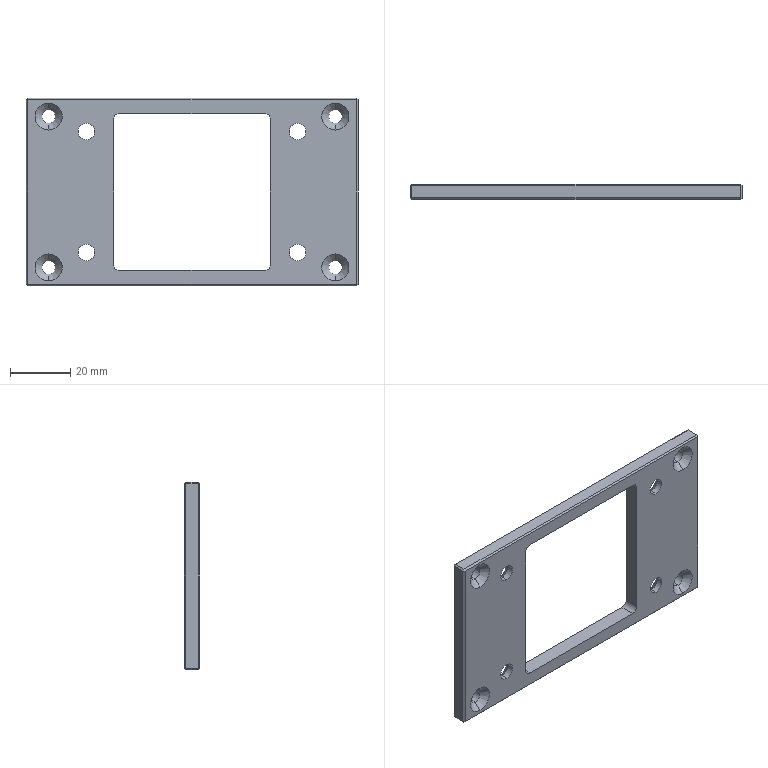Part | STEP file | ND25021-01-JDKM-08-TL | 1 solid | 66 faces | box 110 x 5 x 62 mm | volume 19151 mm3 | plane 30 | cylinder 20 | cone 16 | commonest cylinder face diameters 4.5 x8 5.5 x8 4 x4